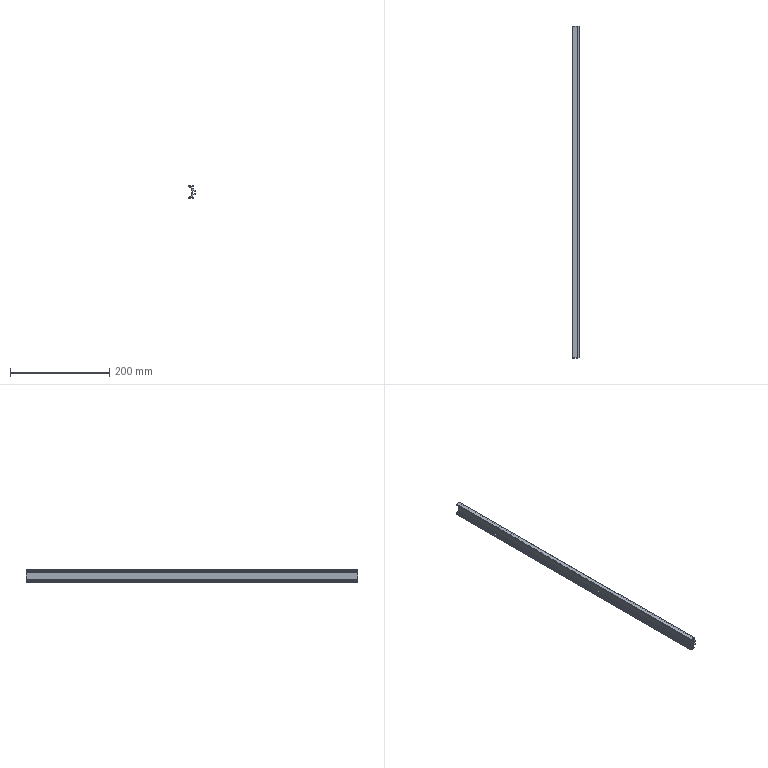Part | STEP file | DEWALT-DWE7492-B22 | 1 solid | 45 faces | box 14 x 670 x 25.488 mm | volume 79850 mm3 | plane 45